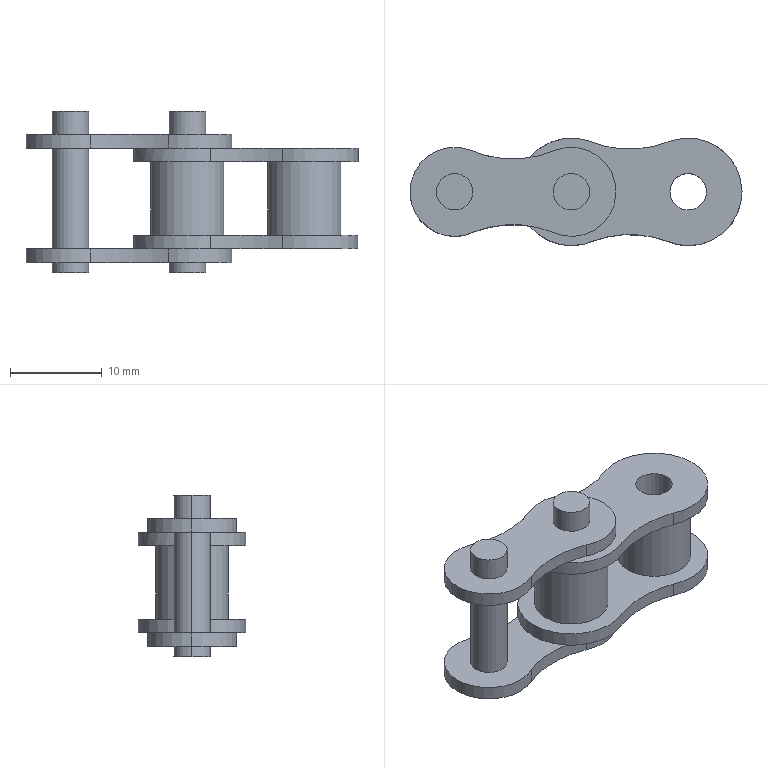Part | STEP file | CHEL40Achain-2 | 1 solid | 48 faces | box 36.1 x 11.7 x 17.55 mm | volume 2131 mm3 | cylinder 36 | plane 12 | commonest cylinder face diameters 3.97 x12 23.4 x8 9.7 x6 11.7 x6 7.95 x4